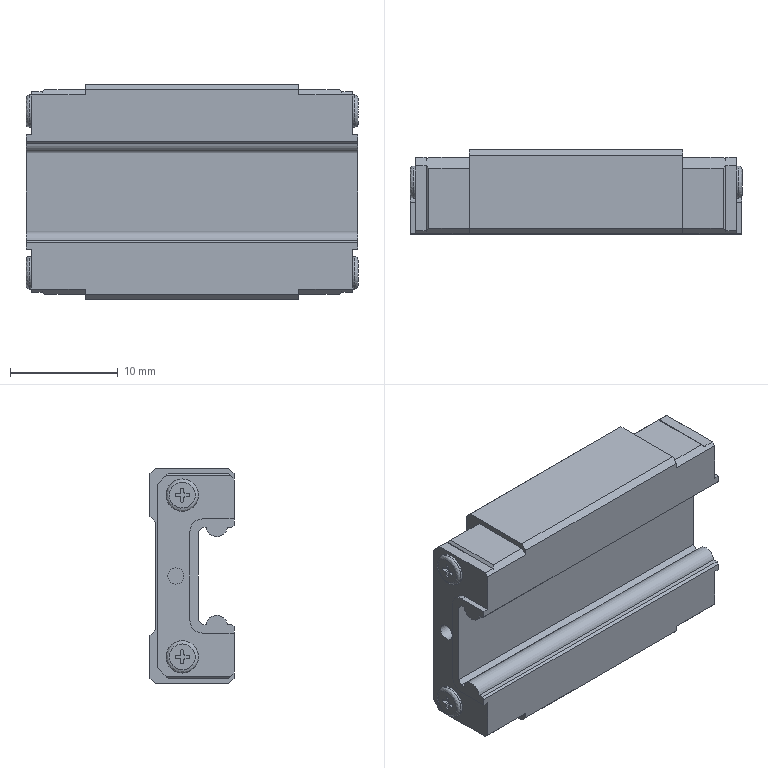Part | STEP file | RSR9KM1-2 | 1 solid | 168 faces | box 30.8 x 7.8 x 20 mm | volume 3450 mm3 | plane 108 | cylinder 48 | cone 8 | spline 4 | commonest cylinder face diameters 0.2 x16 1.3 x16 2.4 x4 2.459 x4 3 x4 1.5 x2